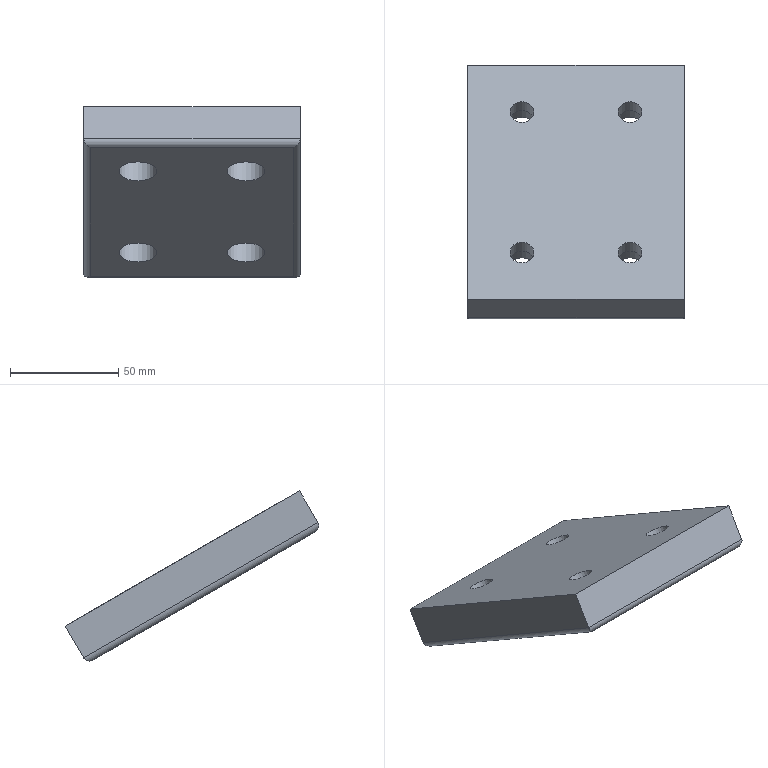Part | NX | features solid 2 | 1 solid | 22 faces | box 100 x 117.155 x 78.722 mm | volume 234555 mm3 | cylinder 12 | plane 10 | commonest cylinder face diameters 6 x4 11 x4 17.5 x4
STEP:
#1=CARTESIAN_POINT('',(185.,910.003,-90.553));
#2=VERTEX_POINT('',#1);
#3=CARTESIAN_POINT('',(185.,918.503,-75.831));
#4=VERTEX_POINT('',#3);
#5=CARTESIAN_POINT('',(185.,913.503,-84.491));
#6=DIRECTION('',(0.,-0.5,-0.866));
#7=VECTOR('',#6,1000.);
#8=LINE('',#5,#7);
#9=EDGE_CURVE('',#2,#4,#8,.F.);
#10=ORIENTED_EDGE('',*,*,#9,.T.);
#11=CARTESIAN_POINT('',(285.,918.503,-75.831));
#12=VERTEX_POINT('',#11);
#13=CARTESIAN_POINT('',(430.,918.503,-75.831));
#14=DIRECTION('',(1.,0.,0.));
#15=VECTOR('',#14,1000.);
#16=LINE('',#13,#15);
#17=EDGE_CURVE('',#4,#12,#16,.T.);
#18=ORIENTED_EDGE('',*,*,#17,.T.);
#19=CARTESIAN_POINT('',(285.,910.003,-90.553));
#20=VERTEX_POINT('',#19);
#21=CARTESIAN_POINT('',(285.,913.503,-84.491));
#22=DIRECTION('',(0.,-0.5,-0.866));
#23=VECTOR('',#22,1000.);
#24=LINE('',#21,#23);
#25=EDGE_CURVE('',#12,#20,#24,.T.);
#26=ORIENTED_EDGE('',*,*,#25,.T.);
#27=CARTESIAN_POINT('',(325.,910.003,-90.553));
#28=DIRECTION('',(1.,0.,0.));
#29=VECTOR('',#28,1000.);
#30=LINE('',#27,#29);
#31=EDGE_CURVE('',#2,#20,#30,.T.);
#32=ORIENTED_EDGE('',*,*,#31,.F.);
#33=EDGE_LOOP('',(#10,#18,#26,#32));
#34=FACE_BOUND('',#33,.T.);
#35=CARTESIAN_POINT('',(325.,908.503,-93.151));
#36=DIRECTION('',(0.,0.866,-0.5));
#37=DIRECTION('',(0.,0.5,0.866));
#38=AXIS2_PLACEMENT_3D('',#35,#36,#37);
#39=PLANE('',#38);
#40=ADVANCED_FACE('',(#34),#39,.T.);
#41=CARTESIAN_POINT('',(285.,801.75,-28.053));
#42=VERTEX_POINT('',#41);
#43=CARTESIAN_POINT('',(285.,810.25,-13.331));
#44=VERTEX_POINT('',#43);
#45=CARTESIAN_POINT('',(285.,800.25,-30.651));
#46=DIRECTION('',(0.,0.5,0.866));
#47=VECTOR('',#46,1000.);
#48=LINE('',#45,#47);
#49=EDGE_CURVE('',#42,#44,#48,.T.);
#50=ORIENTED_EDGE('',*,*,#49,.T.);
#51=CARTESIAN_POINT('',(185.,810.25,-13.331));
#52=VERTEX_POINT('',#51);
#53=CARTESIAN_POINT('',(430.,810.25,-13.331));
#54=DIRECTION('',(1.,0.,0.));
#55=VECTOR('',#54,1000.);
#56=LINE('',#53,#55);
#57=EDGE_CURVE('',#52,#44,#56,.T.);
#58=ORIENTED_EDGE('',*,*,#57,.F.);
#59=CARTESIAN_POINT('',(185.,801.75,-28.053));
#60=VERTEX_POINT('',#59);
#61=CARTESIAN_POINT('',(185.,805.25,-21.991));
#62=DIRECTION('',(0.,-0.5,-0.866));
#63=VECTOR('',#62,1000.);
#64=LINE('',#61,#63);
#65=EDGE_CURVE('',#60,#52,#64,.F.);
#66=ORIENTED_EDGE('',*,*,#65,.F.);
#67=CARTESIAN_POINT('',(430.,801.75,-28.053));
#68=DIRECTION('',(1.,0.,0.));
#69=VECTOR('',#68,1000.);
#70=LINE('',#67,#69);
#71=EDGE_CURVE('',#42,#60,#70,.F.);
#72=ORIENTED_EDGE('',*,*,#71,.F.);
#73=EDGE_LOOP('',(#50,#58,#66,#72));
#74=FACE_BOUND('',#73,.T.);
#75=CARTESIAN_POINT('',(430.,800.25,-30.651));
#76=DIRECTION('',(0.,0.866,-0.5));
#77=DIRECTION('',(0.,0.5,0.866));
#78=AXIS2_PLACEMENT_3D('',#75,#76,#77);
#79=PLANE('',#78);
#80=ADVANCED_FACE('',(#74),#79,.F.);
#81=CARTESIAN_POINT('',(210.,814.323,-38.776));
#82=VERTEX_POINT('',#81);
#83=CARTESIAN_POINT('',(210.,821.901,-43.151));
#84=DIRECTION('',(0.,0.5,0.866));
#85=DIRECTION('',(0.,-0.866,0.5));
#86=AXIS2_PLACEMENT_3D('',#83,#84,#85);
#87=CIRCLE('',#86,8.75);
#88=EDGE_CURVE('',#82,#82,#87,.T.);
#89=ORIENTED_EDGE('',*,*,#88,.T.);
#90=EDGE_LOOP('',(#89));
#91=FACE_BOUND('',#90,.T.);
#92=CARTESIAN_POINT('',(210.,879.275,-76.276));
#93=VERTEX_POINT('',#92);
#94=CARTESIAN_POINT('',(210.,886.853,-80.651));
#95=DIRECTION('',(0.,0.5,0.866));
#96=DIRECTION('',(0.,-0.866,0.5));
#97=AXIS2_PLACEMENT_3D('',#94,#95,#96);
#98=CIRCLE('',#97,8.75);
#99=EDGE_CURVE('',#93,#93,#98,.T.);
#100=ORIENTED_EDGE('',*,*,#99,.T.);
#101=EDGE_LOOP('',(#100));
#102=FACE_BOUND('',#101,.T.);
#103=CARTESIAN_POINT('',(260.,879.275,-76.276));
#104=VERTEX_POINT('',#103);
#105=CARTESIAN_POINT('',(260.,886.853,-80.651));
#106=DIRECTION('',(0.,0.5,0.866));
#107=DIRECTION('',(0.,-0.866,0.5));
#108=AXIS2_PLACEMENT_3D('',#105,#106,#107);
#109=CIRCLE('',#108,8.75);
#110=EDGE_CURVE('',#104,#104,#109,.T.);
#111=ORIENTED_EDGE('',*,*,#110,.T.);
#112=EDGE_LOOP('',(#111));
#113=FACE_BOUND('',#112,.T.);
#114=CARTESIAN_POINT('',(260.,814.323,-38.776));
#115=VERTEX_POINT('',#114);
#116=CARTESIAN_POINT('',(260.,821.901,-43.151));
#117=DIRECTION('',(0.,0.5,0.866));
#118=DIRECTION('',(0.,-0.866,0.5));
#119=AXIS2_PLACEMENT_3D('',#116,#117,#118);
#120=CIRCLE('',#119,8.75);
#121=EDGE_CURVE('',#115,#115,#120,.T.);
#122=ORIENTED_EDGE('',*,*,#121,.T.);
#123=EDGE_LOOP('',(#122));
#124=FACE_BOUND('',#123,.T.);
#125=CARTESIAN_POINT('',(282.,905.905,-91.651));
#126=VERTEX_POINT('',#125);
#127=CARTESIAN_POINT('',(188.,905.905,-91.651));
#128=VERTEX_POINT('',#127);
#129=CARTESIAN_POINT('',(200.,905.905,-91.651));
#130=DIRECTION('',(1.,0.,0.));
#131=VECTOR('',#130,1000.);
#132=LINE('',#129,#131);
#133=EDGE_CURVE('',#126,#128,#132,.F.);
#134=ORIENTED_EDGE('',*,*,#133,.F.);
#135=CARTESIAN_POINT('',(282.,802.848,-32.151));
#136=VERTEX_POINT('',#135);
#137=CARTESIAN_POINT('',(282.,925.824,-103.151));
#138=DIRECTION('',(0.,0.866,-0.5));
#139=VECTOR('',#138,1000.);
#140=LINE('',#137,#139);
#141=EDGE_CURVE('',#126,#136,#140,.F.);
#142=ORIENTED_EDGE('',*,*,#141,.T.);
#143=CARTESIAN_POINT('',(188.,802.848,-32.151));
#144=VERTEX_POINT('',#143);
#145=CARTESIAN_POINT('',(430.,802.848,-32.151));
#146=DIRECTION('',(1.,0.,0.));
#147=VECTOR('',#146,1000.);
#148=LINE('',#145,#147);
#149=EDGE_CURVE('',#144,#136,#148,.T.);
#150=ORIENTED_EDGE('',*,*,#149,.F.);
#151=CARTESIAN_POINT('',(188.,925.824,-103.151));
#152=DIRECTION('',(0.,0.866,-0.5));
#153=VECTOR('',#152,1000.);
#154=LINE('',#151,#153);
#155=EDGE_CURVE('',#128,#144,#154,.F.);
#156=ORIENTED_EDGE('',*,*,#155,.F.);
#157=EDGE_LOOP('',(#134,#142,#150,#156));
#158=FACE_BOUND('',#157,.T.);
#159=CARTESIAN_POINT('',(430.,925.824,-103.151));
#160=DIRECTION('',(0.,0.5,0.866));
#161=DIRECTION('',(0.,0.866,-0.5));
#162=AXIS2_PLACEMENT_3D('',#159,#160,#161);
#163=PLANE('',#162);
#164=ADVANCED_FACE('',(#91,#102,#113,#124,#158),#163,.F.);
#165=CARTESIAN_POINT('',(210.,827.137,-23.081));
#166=VERTEX_POINT('',#165);
#167=CARTESIAN_POINT('',(210.,831.901,-25.831));
#168=DIRECTION('',(0.,0.5,0.866));
#169=DIRECTION('',(0.,-0.866,0.5));
#170=AXIS2_PLACEMENT_3D('',#167,#168,#169);
#171=CIRCLE('',#170,5.5);
#172=EDGE_CURVE('',#166,#166,#171,.T.);
#173=ORIENTED_EDGE('',*,*,#172,.F.);
#174=EDGE_LOOP('',(#173));
#175=FACE_BOUND('',#174,.T.);
#176=CARTESIAN_POINT('',(210.,892.089,-60.581));
#177=VERTEX_POINT('',#176);
#178=CARTESIAN_POINT('',(210.,896.853,-63.331));
#179=DIRECTION('',(0.,0.5,0.866));
#180=DIRECTION('',(0.,-0.866,0.5));
#181=AXIS2_PLACEMENT_3D('',#178,#179,#180);
#182=CIRCLE('',#181,5.5);
#183=EDGE_CURVE('',#177,#177,#182,.T.);
#184=ORIENTED_EDGE('',*,*,#183,.F.);
#185=EDGE_LOOP('',(#184));
#186=FACE_BOUND('',#185,.T.);
#187=CARTESIAN_POINT('',(260.,892.089,-60.581));
#188=VERTEX_POINT('',#187);
#189=CARTESIAN_POINT('',(260.,896.853,-63.331));
#190=DIRECTION('',(0.,0.5,0.866));
#191=DIRECTION('',(0.,-0.866,0.5));
#192=AXIS2_PLACEMENT_3D('',#189,#190,#191);
#193=CIRCLE('',#192,5.5);
#194=EDGE_CURVE('',#188,#188,#193,.T.);
#195=ORIENTED_EDGE('',*,*,#194,.F.);
#196=EDGE_LOOP('',(#195));
#197=FACE_BOUND('',#196,.T.);
#198=CARTESIAN_POINT('',(260.,827.137,-23.081));
#199=VERTEX_POINT('',#198);
#200=CARTESIAN_POINT('',(260.,831.901,-25.831));
#201=DIRECTION('',(0.,0.5,0.866));
#202=DIRECTION('',(0.,-0.866,0.5));
#203=AXIS2_PLACEMENT_3D('',#200,#201,#202);
#204=CIRCLE('',#203,5.5);
#205=EDGE_CURVE('',#199,#199,#204,.T.);
#206=ORIENTED_EDGE('',*,*,#205,.F.);
#207=EDGE_LOOP('',(#206));
#208=FACE_BOUND('',#207,.T.);
#209=CARTESIAN_POINT('',(185.,935.824,-85.831));
#210=DIRECTION('',(0.,-0.866,0.5));
#211=VECTOR('',#210,1000.);
#212=LINE('',#209,#211);
#213=EDGE_CURVE('',#52,#4,#212,.F.);
#214=ORIENTED_EDGE('',*,*,#213,.F.);
#215=ORIENTED_EDGE('',*,*,#57,.T.);
#216=CARTESIAN_POINT('',(285.,935.824,-85.831));
#217=DIRECTION('',(0.,-0.866,0.5));
#218=VECTOR('',#217,1000.);
#219=LINE('',#216,#218);
#220=EDGE_CURVE('',#12,#44,#219,.T.);
#221=ORIENTED_EDGE('',*,*,#220,.F.);
#222=ORIENTED_EDGE('',*,*,#17,.F.);
#223=EDGE_LOOP('',(#214,#215,#221,#222));
#224=FACE_BOUND('',#223,.T.);
#225=CARTESIAN_POINT('',(430.,935.824,-85.831));
#226=DIRECTION('',(0.,0.5,0.866));
#227=DIRECTION('',(0.,0.866,-0.5));
#228=AXIS2_PLACEMENT_3D('',#225,#226,#227);
#229=PLANE('',#228);
#230=ADVANCED_FACE('',(#175,#186,#197,#208,#224),#229,.T.);
#231=ORIENTED_EDGE('',*,*,#65,.T.);
#232=ORIENTED_EDGE('',*,*,#213,.T.);
#233=ORIENTED_EDGE('',*,*,#9,.F.);
#234=CARTESIAN_POINT('',(185.,927.324,-100.553));
#235=DIRECTION('',(0.,-0.866,0.5));
#236=VECTOR('',#235,1000.);
#237=LINE('',#234,#236);
#238=EDGE_CURVE('',#60,#2,#237,.F.);
#239=ORIENTED_EDGE('',*,*,#238,.F.);
#240=EDGE_LOOP('',(#231,#232,#233,#239));
#241=FACE_BOUND('',#240,.T.);
#242=CARTESIAN_POINT('',(185.,1013.096,-141.991));
#243=DIRECTION('',(1.,0.,0.));
#244=DIRECTION('',(0.,-1.,0.));
#245=AXIS2_PLACEMENT_3D('',#242,#243,#244);
#246=PLANE('',#245);
#247=ADVANCED_FACE('',(#241),#246,.F.);
#248=ORIENTED_EDGE('',*,*,#49,.F.);
#249=CARTESIAN_POINT('',(285.,1009.596,-148.053));
#250=DIRECTION('',(0.,0.866,-0.5));
#251=VECTOR('',#250,1000.);
#252=LINE('',#249,#251);
#253=EDGE_CURVE('',#42,#20,#252,.T.);
#254=ORIENTED_EDGE('',*,*,#253,.T.);
#255=ORIENTED_EDGE('',*,*,#25,.F.);
#256=ORIENTED_EDGE('',*,*,#220,.T.);
#257=EDGE_LOOP('',(#248,#254,#255,#256));
#258=FACE_BOUND('',#257,.T.);
#259=CARTESIAN_POINT('',(285.,1013.096,-141.991));
#260=DIRECTION('',(1.,0.,0.));
#261=DIRECTION('',(0.,-1.,0.));
#262=AXIS2_PLACEMENT_3D('',#259,#260,#261);
#263=PLANE('',#262);
#264=ADVANCED_FACE('',(#258),#263,.T.);
#265=ORIENTED_EDGE('',*,*,#149,.T.);
#266=CARTESIAN_POINT('',(282.,804.348,-29.553));
#267=DIRECTION('',(-0.7071,-0.6124,0.3536));
#268=DIRECTION('',(-0.7071,0.6124,-0.3536));
#269=AXIS2_PLACEMENT_3D('',#266,#267,#268);
#270=ELLIPSE('',#269,4.243,3.);
#271=EDGE_CURVE('',#136,#42,#270,.T.);
#272=ORIENTED_EDGE('',*,*,#271,.T.);
#273=ORIENTED_EDGE('',*,*,#71,.T.);
#274=CARTESIAN_POINT('',(188.,804.348,-29.553));
#275=DIRECTION('',(-0.7071,0.6124,-0.3536));
#276=DIRECTION('',(-0.7071,-0.6124,0.3536));
#277=AXIS2_PLACEMENT_3D('',#274,#275,#276);
#278=ELLIPSE('',#277,4.243,3.);
#279=EDGE_CURVE('',#60,#144,#278,.F.);
#280=ORIENTED_EDGE('',*,*,#279,.T.);
#281=EDGE_LOOP('',(#265,#272,#273,#280));
#282=FACE_BOUND('',#281,.T.);
#283=CARTESIAN_POINT('',(430.,804.348,-29.553));
#284=DIRECTION('',(1.,0.,0.));
#285=DIRECTION('',(0.,0.,1.));
#286=AXIS2_PLACEMENT_3D('',#283,#284,#285);
#287=CYLINDRICAL_SURFACE('',#286,3.);
#288=ADVANCED_FACE('',(#282),#287,.T.);
#289=ORIENTED_EDGE('',*,*,#31,.T.);
#290=CARTESIAN_POINT('',(282.,907.405,-89.053));
#291=DIRECTION('',(0.7071,-0.6124,0.3536));
#292=DIRECTION('',(0.7071,0.6124,-0.3536));
#293=AXIS2_PLACEMENT_3D('',#290,#291,#292);
#294=ELLIPSE('',#293,4.243,3.);
#295=EDGE_CURVE('',#20,#126,#294,.F.);
#296=ORIENTED_EDGE('',*,*,#295,.T.);
#297=ORIENTED_EDGE('',*,*,#133,.T.);
#298=CARTESIAN_POINT('',(188.,907.405,-89.053));
#299=DIRECTION('',(0.7071,0.6124,-0.3536));
#300=DIRECTION('',(0.7071,-0.6124,0.3536));
#301=AXIS2_PLACEMENT_3D('',#298,#299,#300);
#302=ELLIPSE('',#301,4.243,3.);
#303=EDGE_CURVE('',#128,#2,#302,.T.);
#304=ORIENTED_EDGE('',*,*,#303,.T.);
#305=EDGE_LOOP('',(#289,#296,#297,#304));
#306=FACE_BOUND('',#305,.T.);
#307=CARTESIAN_POINT('',(325.,907.405,-89.053));
#308=DIRECTION('',(-1.,0.,0.));
#309=DIRECTION('',(0.,0.,-1.));
#310=AXIS2_PLACEMENT_3D('',#307,#308,#309);
#311=CYLINDRICAL_SURFACE('',#310,3.);
#312=ADVANCED_FACE('',(#306),#311,.T.);
#313=ORIENTED_EDGE('',*,*,#279,.F.);
#314=ORIENTED_EDGE('',*,*,#238,.T.);
#315=ORIENTED_EDGE('',*,*,#303,.F.);
#316=ORIENTED_EDGE('',*,*,#155,.T.);
#317=EDGE_LOOP('',(#313,#314,#315,#316));
#318=FACE_BOUND('',#317,.T.);
#319=CARTESIAN_POINT('',(188.,927.324,-100.553));
#320=DIRECTION('',(0.,-0.866,0.5));
#321=DIRECTION('',(0.,-0.5,-0.866));
#322=AXIS2_PLACEMENT_3D('',#319,#320,#321);
#323=CYLINDRICAL_SURFACE('',#322,3.);
#324=ADVANCED_FACE('',(#318),#323,.T.);
#325=ORIENTED_EDGE('',*,*,#271,.F.);
#326=ORIENTED_EDGE('',*,*,#141,.F.);
#327=ORIENTED_EDGE('',*,*,#295,.F.);
#328=ORIENTED_EDGE('',*,*,#253,.F.);
#329=EDGE_LOOP('',(#325,#326,#327,#328));
#330=FACE_BOUND('',#329,.T.);
#331=CARTESIAN_POINT('',(282.,1009.596,-148.053));
#332=DIRECTION('',(0.,0.866,-0.5));
#333=DIRECTION('',(0.,0.5,0.866));
#334=AXIS2_PLACEMENT_3D('',#331,#332,#333);
#335=CYLINDRICAL_SURFACE('',#334,3.);
#336=ADVANCED_FACE('',(#330),#335,.T.);
#337=ORIENTED_EDGE('',*,*,#205,.T.);
#338=EDGE_LOOP('',(#337));
#339=FACE_BOUND('',#338,.T.);
#340=CARTESIAN_POINT('',(260.,823.137,-30.009));
#341=VERTEX_POINT('',#340);
#342=CARTESIAN_POINT('',(260.,827.901,-32.759));
#343=DIRECTION('',(0.,0.5,0.866));
#344=DIRECTION('',(0.,-0.866,0.5));
#345=AXIS2_PLACEMENT_3D('',#342,#343,#344);
#346=CIRCLE('',#345,5.5);
#347=EDGE_CURVE('',#341,#341,#346,.T.);
#348=ORIENTED_EDGE('',*,*,#347,.F.);
#349=EDGE_LOOP('',(#348));
#350=FACE_BOUND('',#349,.T.);
#351=CARTESIAN_POINT('',(260.,871.901,43.451));
#352=DIRECTION('',(0.,0.5,0.866));
#353=DIRECTION('',(0.,-0.866,0.5));
#354=AXIS2_PLACEMENT_3D('',#351,#352,#353);
#355=CYLINDRICAL_SURFACE('',#354,5.5);
#356=ADVANCED_FACE('',(#339,#350),#355,.F.);
#357=ORIENTED_EDGE('',*,*,#347,.T.);
#358=EDGE_LOOP('',(#357));
#359=FACE_BOUND('',#358,.T.);
#360=CARTESIAN_POINT('',(260.,820.323,-28.384));
#361=VERTEX_POINT('',#360);
#362=CARTESIAN_POINT('',(260.,827.901,-32.759));
#363=DIRECTION('',(0.,0.5,0.866));
#364=DIRECTION('',(0.,-0.866,0.5));
#365=AXIS2_PLACEMENT_3D('',#362,#363,#364);
#366=CIRCLE('',#365,8.75);
#367=EDGE_CURVE('',#361,#361,#366,.T.);
#368=ORIENTED_EDGE('',*,*,#367,.F.);
#369=EDGE_LOOP('',(#368));
#370=FACE_BOUND('',#369,.T.);
#371=CARTESIAN_POINT('',(260.,827.901,-32.759));
#372=DIRECTION('',(0.,0.5,0.866));
#373=DIRECTION('',(0.,-0.866,0.5));
#374=AXIS2_PLACEMENT_3D('',#371,#372,#373);
#375=PLANE('',#374);
#376=ADVANCED_FACE('',(#359,#370),#375,.F.);
#377=ORIENTED_EDGE('',*,*,#367,.T.);
#378=EDGE_LOOP('',(#377));
#379=FACE_BOUND('',#378,.T.);
#380=ORIENTED_EDGE('',*,*,#121,.F.);
#381=EDGE_LOOP('',(#380));
#382=FACE_BOUND('',#381,.T.);
#383=CARTESIAN_POINT('',(260.,821.901,-43.151));
#384=DIRECTION('',(0.,0.5,0.866));
#385=DIRECTION('',(0.,-0.866,0.5));
#386=AXIS2_PLACEMENT_3D('',#383,#384,#385);
#387=CYLINDRICAL_SURFACE('',#386,8.75);
#388=ADVANCED_FACE('',(#379,#382),#387,.F.);
#389=ORIENTED_EDGE('',*,*,#194,.T.);
#390=EDGE_LOOP('',(#389));
#391=FACE_BOUND('',#390,.T.);
#392=CARTESIAN_POINT('',(260.,888.089,-67.509));
#393=VERTEX_POINT('',#392);
#394=CARTESIAN_POINT('',(260.,892.853,-70.259));
#395=DIRECTION('',(0.,0.5,0.866));
#396=DIRECTION('',(0.,-0.866,0.5));
#397=AXIS2_PLACEMENT_3D('',#394,#395,#396);
#398=CIRCLE('',#397,5.5);
#399=EDGE_CURVE('',#393,#393,#398,.T.);
#400=ORIENTED_EDGE('',*,*,#399,.F.);
#401=EDGE_LOOP('',(#400));
#402=FACE_BOUND('',#401,.T.);
#403=CARTESIAN_POINT('',(260.,936.853,5.951));
#404=DIRECTION('',(0.,0.5,0.866));
#405=DIRECTION('',(0.,-0.866,0.5));
#406=AXIS2_PLACEMENT_3D('',#403,#404,#405);
#407=CYLINDRICAL_SURFACE('',#406,5.5);
#408=ADVANCED_FACE('',(#391,#402),#407,.F.);
#409=ORIENTED_EDGE('',*,*,#399,.T.);
#410=EDGE_LOOP('',(#409));
#411=FACE_BOUND('',#410,.T.);
#412=CARTESIAN_POINT('',(260.,885.275,-65.884));
#413=VERTEX_POINT('',#412);
#414=CARTESIAN_POINT('',(260.,892.853,-70.259));
#415=DIRECTION('',(0.,0.5,0.866));
#416=DIRECTION('',(0.,-0.866,0.5));
#417=AXIS2_PLACEMENT_3D('',#414,#415,#416);
#418=CIRCLE('',#417,8.75);
#419=EDGE_CURVE('',#413,#413,#418,.T.);
#420=ORIENTED_EDGE('',*,*,#419,.F.);
#421=EDGE_LOOP('',(#420));
#422=FACE_BOUND('',#421,.T.);
#423=CARTESIAN_POINT('',(260.,892.853,-70.259));
#424=DIRECTION('',(0.,0.5,0.866));
#425=DIRECTION('',(0.,-0.866,0.5));
#426=AXIS2_PLACEMENT_3D('',#423,#424,#425);
#427=PLANE('',#426);
#428=ADVANCED_FACE('',(#411,#422),#427,.F.);
#429=ORIENTED_EDGE('',*,*,#419,.T.);
#430=EDGE_LOOP('',(#429));
#431=FACE_BOUND('',#430,.T.);
#432=ORIENTED_EDGE('',*,*,#110,.F.);
#433=EDGE_LOOP('',(#432));
#434=FACE_BOUND('',#433,.T.);
#435=CARTESIAN_POINT('',(260.,886.853,-80.651));
#436=DIRECTION('',(0.,0.5,0.866));
#437=DIRECTION('',(0.,-0.866,0.5));
#438=AXIS2_PLACEMENT_3D('',#435,#436,#437);
#439=CYLINDRICAL_SURFACE('',#438,8.75);
#440=ADVANCED_FACE('',(#431,#434),#439,.F.);
#441=ORIENTED_EDGE('',*,*,#183,.T.);
#442=EDGE_LOOP('',(#441));
#443=FACE_BOUND('',#442,.T.);
#444=CARTESIAN_POINT('',(210.,888.089,-67.509));
#445=VERTEX_POINT('',#444);
#446=CARTESIAN_POINT('',(210.,892.853,-70.259));
#447=DIRECTION('',(0.,0.5,0.866));
#448=DIRECTION('',(0.,-0.866,0.5));
#449=AXIS2_PLACEMENT_3D('',#446,#447,#448);
#450=CIRCLE('',#449,5.5);
#451=EDGE_CURVE('',#445,#445,#450,.T.);
#452=ORIENTED_EDGE('',*,*,#451,.F.);
#453=EDGE_LOOP('',(#452));
#454=FACE_BOUND('',#453,.T.);
#455=CARTESIAN_POINT('',(210.,936.853,5.951));
#456=DIRECTION('',(0.,0.5,0.866));
#457=DIRECTION('',(0.,-0.866,0.5));
#458=AXIS2_PLACEMENT_3D('',#455,#456,#457);
#459=CYLINDRICAL_SURFACE('',#458,5.5);
#460=ADVANCED_FACE('',(#443,#454),#459,.F.);
#461=ORIENTED_EDGE('',*,*,#451,.T.);
#462=EDGE_LOOP('',(#461));
#463=FACE_BOUND('',#462,.T.);
#464=CARTESIAN_POINT('',(210.,885.275,-65.884));
#465=VERTEX_POINT('',#464);
#466=CARTESIAN_POINT('',(210.,892.853,-70.259));
#467=DIRECTION('',(0.,0.5,0.866));
#468=DIRECTION('',(0.,-0.866,0.5));
#469=AXIS2_PLACEMENT_3D('',#466,#467,#468);
#470=CIRCLE('',#469,8.75);
#471=EDGE_CURVE('',#465,#465,#470,.T.);
#472=ORIENTED_EDGE('',*,*,#471,.F.);
#473=EDGE_LOOP('',(#472));
#474=FACE_BOUND('',#473,.T.);
#475=CARTESIAN_POINT('',(210.,892.853,-70.259));
#476=DIRECTION('',(0.,0.5,0.866));
#477=DIRECTION('',(0.,-0.866,0.5));
#478=AXIS2_PLACEMENT_3D('',#475,#476,#477);
#479=PLANE('',#478);
#480=ADVANCED_FACE('',(#463,#474),#479,.F.);
#481=ORIENTED_EDGE('',*,*,#471,.T.);
#482=EDGE_LOOP('',(#481));
#483=FACE_BOUND('',#482,.T.);
#484=ORIENTED_EDGE('',*,*,#99,.F.);
#485=EDGE_LOOP('',(#484));
#486=FACE_BOUND('',#485,.T.);
#487=CARTESIAN_POINT('',(210.,886.853,-80.651));
#488=DIRECTION('',(0.,0.5,0.866));
#489=DIRECTION('',(0.,-0.866,0.5));
#490=AXIS2_PLACEMENT_3D('',#487,#488,#489);
#491=CYLINDRICAL_SURFACE('',#490,8.75);
#492=ADVANCED_FACE('',(#483,#486),#491,.F.);
#493=ORIENTED_EDGE('',*,*,#172,.T.);
#494=EDGE_LOOP('',(#493));
#495=FACE_BOUND('',#494,.T.);
#496=CARTESIAN_POINT('',(210.,823.137,-30.009));
#497=VERTEX_POINT('',#496);
#498=CARTESIAN_POINT('',(210.,827.901,-32.759));
#499=DIRECTION('',(0.,0.5,0.866));
#500=DIRECTION('',(0.,-0.866,0.5));
#501=AXIS2_PLACEMENT_3D('',#498,#499,#500);
#502=CIRCLE('',#501,5.5);
#503=EDGE_CURVE('',#497,#497,#502,.T.);
#504=ORIENTED_EDGE('',*,*,#503,.F.);
#505=EDGE_LOOP('',(#504));
#506=FACE_BOUND('',#505,.T.);
#507=CARTESIAN_POINT('',(210.,871.901,43.451));
#508=DIRECTION('',(0.,0.5,0.866));
#509=DIRECTION('',(0.,-0.866,0.5));
#510=AXIS2_PLACEMENT_3D('',#507,#508,#509);
#511=CYLINDRICAL_SURFACE('',#510,5.5);
#512=ADVANCED_FACE('',(#495,#506),#511,.F.);
#513=ORIENTED_EDGE('',*,*,#503,.T.);
#514=EDGE_LOOP('',(#513));
#515=FACE_BOUND('',#514,.T.);
#516=CARTESIAN_POINT('',(210.,820.323,-28.384));
#517=VERTEX_POINT('',#516);
#518=CARTESIAN_POINT('',(210.,827.901,-32.759));
#519=DIRECTION('',(0.,0.5,0.866));
#520=DIRECTION('',(0.,-0.866,0.5));
#521=AXIS2_PLACEMENT_3D('',#518,#519,#520);
#522=CIRCLE('',#521,8.75);
#523=EDGE_CURVE('',#517,#517,#522,.T.);
#524=ORIENTED_EDGE('',*,*,#523,.F.);
#525=EDGE_LOOP('',(#524));
#526=FACE_BOUND('',#525,.T.);
#527=CARTESIAN_POINT('',(210.,827.901,-32.759));
#528=DIRECTION('',(0.,0.5,0.866));
#529=DIRECTION('',(0.,-0.866,0.5));
#530=AXIS2_PLACEMENT_3D('',#527,#528,#529);
#531=PLANE('',#530);
#532=ADVANCED_FACE('',(#515,#526),#531,.F.);
#533=ORIENTED_EDGE('',*,*,#523,.T.);
#534=EDGE_LOOP('',(#533));
#535=FACE_BOUND('',#534,.T.);
#536=ORIENTED_EDGE('',*,*,#88,.F.);
#537=EDGE_LOOP('',(#536));
#538=FACE_BOUND('',#537,.T.);
#539=CARTESIAN_POINT('',(210.,821.901,-43.151));
#540=DIRECTION('',(0.,0.5,0.866));
#541=DIRECTION('',(0.,-0.866,0.5));
#542=AXIS2_PLACEMENT_3D('',#539,#540,#541);
#543=CYLINDRICAL_SURFACE('',#542,8.75);
#544=ADVANCED_FACE('',(#535,#538),#543,.F.);
#545=CLOSED_SHELL('',(#40,#80,#164,#230,#247,#264,#288,#312,#324,#336,#356,#376,#388,#408,#428,#440,#460,#480,#492,#512,#532,#544));
#546=MANIFOLD_SOLID_BREP('',#545);
#547=(LENGTH_UNIT()NAMED_UNIT(*)SI_UNIT(.MILLI.,.METRE.));
#548=UNCERTAINTY_MEASURE_WITH_UNIT(LENGTH_MEASURE(0.00001),#547,'','');
#549=(NAMED_UNIT(*)PLANE_ANGLE_UNIT()SI_UNIT($,.RADIAN.));
#550=(NAMED_UNIT(*)SI_UNIT($,.STERADIAN.)SOLID_ANGLE_UNIT());
#551=(GEOMETRIC_REPRESENTATION_CONTEXT(3)GLOBAL_UNCERTAINTY_ASSIGNED_CONTEXT((#548))GLOBAL_UNIT_ASSIGNED_CONTEXT((#547,#549,#550))REPRESENTATION_CONTEXT('',''));
#552=ADVANCED_BREP_SHAPE_REPRESENTATION('',(#546),#551);